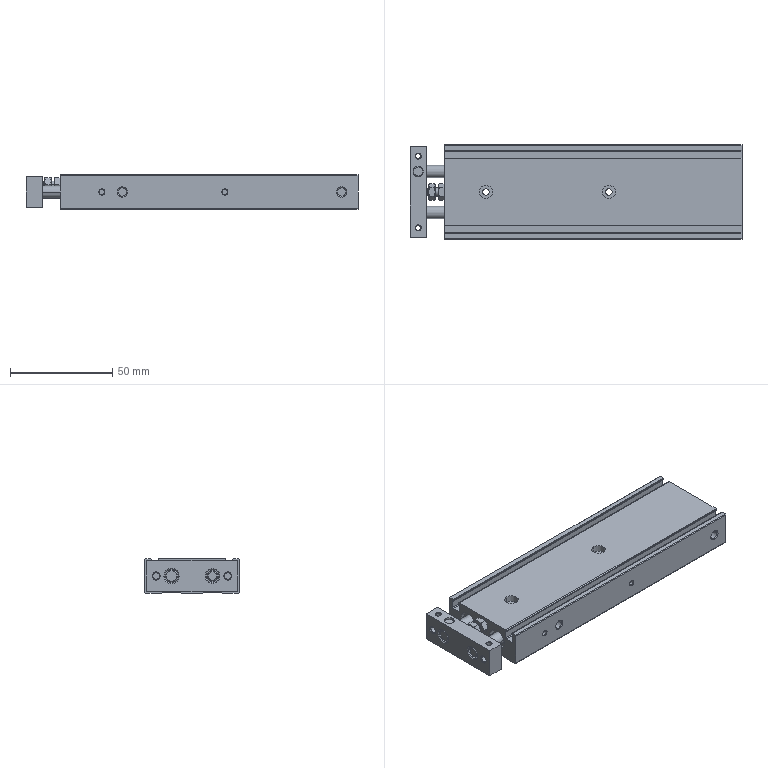Part | STEP file | 2 solids | 251 faces | box 162 x 46 x 17 mm | volume 100309 mm3 | cylinder 94 | plane 81 | cone 76 | commonest cylinder face diameters 2.459 x16 10 x16 0.8 x12 6 x10 3.242 x8 4.134 x8